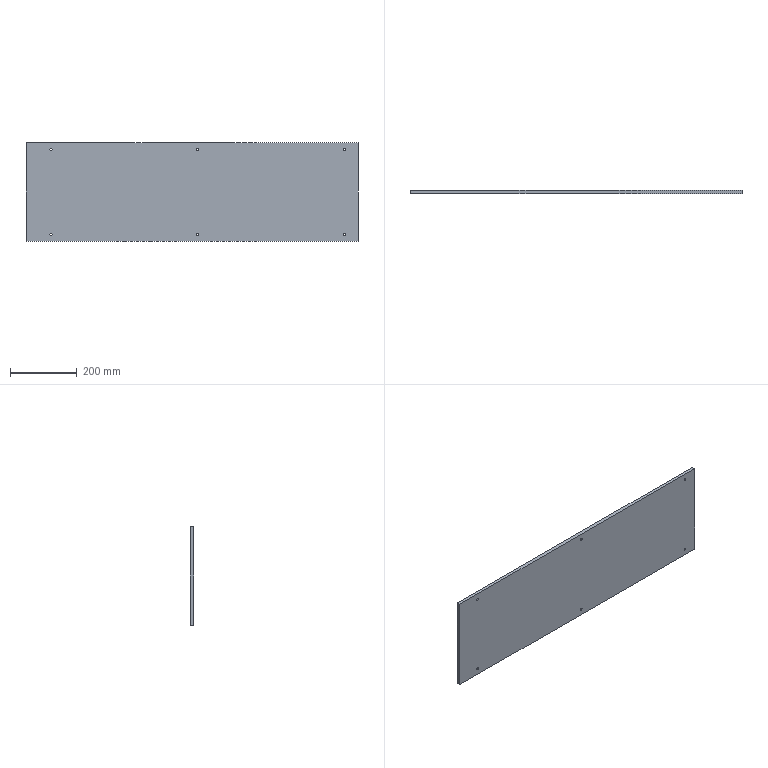Part | SolidWorks | features Extrusion 1, HoleWzd 1 | 1 solid | 30 faces | box 995 x 10 x 295 mm | volume 2932412 mm3 | cone 12 | cylinder 12 | plane 6 | commonest cylinder face diameters 6.6 x12
STEP:
#1=CARTESIAN_POINT('',(75.,6.9,16.7));
#2=VERTEX_POINT('',#1);
#3=CARTESIAN_POINT('',(75.,6.9,23.3));
#4=VERTEX_POINT('',#3);
#5=CARTESIAN_POINT('',(75.,6.9,20.));
#6=DIRECTION('',(0.,1.,0.));
#7=DIRECTION('',(0.,0.,1.));
#8=AXIS2_PLACEMENT_3D('',#5,#6,#7);
#9=CIRCLE('',#8,3.3);
#10=EDGE_CURVE('',#2,#4,#9,.T.);
#11=ORIENTED_EDGE('',*,*,#10,.F.);
#12=CARTESIAN_POINT('',(75.,10.,13.6));
#13=VERTEX_POINT('',#12);
#14=CARTESIAN_POINT('',(75.,10.,13.6));
#15=DIRECTION('',(0.,0.7071,-0.7071));
#16=VECTOR('',#15,1000.);
#17=LINE('',#14,#16);
#18=EDGE_CURVE('',#2,#13,#17,.T.);
#19=ORIENTED_EDGE('',*,*,#18,.T.);
#20=CARTESIAN_POINT('',(75.,10.,26.4));
#21=VERTEX_POINT('',#20);
#22=CARTESIAN_POINT('',(75.,10.,20.));
#23=DIRECTION('',(0.,1.,0.));
#24=DIRECTION('',(0.,0.,1.));
#25=AXIS2_PLACEMENT_3D('',#22,#23,#24);
#26=CIRCLE('',#25,6.4);
#27=EDGE_CURVE('',#13,#21,#26,.T.);
#28=ORIENTED_EDGE('',*,*,#27,.T.);
#29=CARTESIAN_POINT('',(75.,10.,26.4));
#30=DIRECTION('',(0.,0.7071,0.7071));
#31=VECTOR('',#30,1000.);
#32=LINE('',#29,#31);
#33=EDGE_CURVE('',#4,#21,#32,.T.);
#34=ORIENTED_EDGE('',*,*,#33,.F.);
#35=EDGE_LOOP('',(#11,#19,#28,#34));
#36=FACE_OUTER_BOUND('',#35,.T.);
#37=CARTESIAN_POINT('',(75.,10.,20.));
#38=DIRECTION('',(0.,1.,0.));
#39=DIRECTION('',(0.,0.,1.));
#40=AXIS2_PLACEMENT_3D('',#37,#38,#39);
#41=CONICAL_SURFACE('',#40,6.4,0.7854);
#42=ADVANCED_FACE('',(#36),#41,.F.);
#43=CARTESIAN_POINT('',(75.,0.,16.7));
#44=VERTEX_POINT('',#43);
#45=CARTESIAN_POINT('',(75.,0.,23.3));
#46=VERTEX_POINT('',#45);
#47=CARTESIAN_POINT('',(75.,0.,20.));
#48=DIRECTION('',(0.,1.,0.));
#49=DIRECTION('',(0.,0.,1.));
#50=AXIS2_PLACEMENT_3D('',#47,#48,#49);
#51=CIRCLE('',#50,3.3);
#52=EDGE_CURVE('',#44,#46,#51,.T.);
#53=ORIENTED_EDGE('',*,*,#52,.F.);
#54=CARTESIAN_POINT('',(75.,10.,16.7));
#55=DIRECTION('',(0.,1.,0.));
#56=VECTOR('',#55,1000.);
#57=LINE('',#54,#56);
#58=EDGE_CURVE('',#44,#2,#57,.T.);
#59=ORIENTED_EDGE('',*,*,#58,.T.);
#60=ORIENTED_EDGE('',*,*,#10,.T.);
#61=CARTESIAN_POINT('',(75.,10.,23.3));
#62=DIRECTION('',(0.,1.,0.));
#63=VECTOR('',#62,1000.);
#64=LINE('',#61,#63);
#65=EDGE_CURVE('',#46,#4,#64,.T.);
#66=ORIENTED_EDGE('',*,*,#65,.F.);
#67=EDGE_LOOP('',(#53,#59,#60,#66));
#68=FACE_OUTER_BOUND('',#67,.T.);
#69=CARTESIAN_POINT('',(75.,10.,20.));
#70=DIRECTION('',(0.,1.,0.));
#71=DIRECTION('',(0.,0.,1.));
#72=AXIS2_PLACEMENT_3D('',#69,#70,#71);
#73=CYLINDRICAL_SURFACE('',#72,3.3);
#74=ADVANCED_FACE('',(#68),#73,.F.);
#75=CARTESIAN_POINT('',(75.,6.9,271.7));
#76=VERTEX_POINT('',#75);
#77=CARTESIAN_POINT('',(75.,6.9,278.3));
#78=VERTEX_POINT('',#77);
#79=CARTESIAN_POINT('',(75.,6.9,275.));
#80=DIRECTION('',(0.,1.,0.));
#81=DIRECTION('',(0.,0.,1.));
#82=AXIS2_PLACEMENT_3D('',#79,#80,#81);
#83=CIRCLE('',#82,3.3);
#84=EDGE_CURVE('',#76,#78,#83,.T.);
#85=ORIENTED_EDGE('',*,*,#84,.F.);
#86=CARTESIAN_POINT('',(75.,10.,268.6));
#87=VERTEX_POINT('',#86);
#88=CARTESIAN_POINT('',(75.,10.,268.6));
#89=DIRECTION('',(0.,0.7071,-0.7071));
#90=VECTOR('',#89,1000.);
#91=LINE('',#88,#90);
#92=EDGE_CURVE('',#76,#87,#91,.T.);
#93=ORIENTED_EDGE('',*,*,#92,.T.);
#94=CARTESIAN_POINT('',(75.,10.,281.4));
#95=VERTEX_POINT('',#94);
#96=CARTESIAN_POINT('',(75.,10.,275.));
#97=DIRECTION('',(0.,1.,0.));
#98=DIRECTION('',(0.,0.,1.));
#99=AXIS2_PLACEMENT_3D('',#96,#97,#98);
#100=CIRCLE('',#99,6.4);
#101=EDGE_CURVE('',#87,#95,#100,.T.);
#102=ORIENTED_EDGE('',*,*,#101,.T.);
#103=CARTESIAN_POINT('',(75.,10.,281.4));
#104=DIRECTION('',(0.,0.7071,0.7071));
#105=VECTOR('',#104,1000.);
#106=LINE('',#103,#105);
#107=EDGE_CURVE('',#78,#95,#106,.T.);
#108=ORIENTED_EDGE('',*,*,#107,.F.);
#109=EDGE_LOOP('',(#85,#93,#102,#108));
#110=FACE_OUTER_BOUND('',#109,.T.);
#111=CARTESIAN_POINT('',(75.,10.,275.));
#112=DIRECTION('',(0.,1.,0.));
#113=DIRECTION('',(0.,0.,1.));
#114=AXIS2_PLACEMENT_3D('',#111,#112,#113);
#115=CONICAL_SURFACE('',#114,6.4,0.7854);
#116=ADVANCED_FACE('',(#110),#115,.F.);
#117=CARTESIAN_POINT('',(75.,0.,271.7));
#118=VERTEX_POINT('',#117);
#119=CARTESIAN_POINT('',(75.,0.,278.3));
#120=VERTEX_POINT('',#119);
#121=CARTESIAN_POINT('',(75.,0.,275.));
#122=DIRECTION('',(0.,1.,0.));
#123=DIRECTION('',(0.,0.,1.));
#124=AXIS2_PLACEMENT_3D('',#121,#122,#123);
#125=CIRCLE('',#124,3.3);
#126=EDGE_CURVE('',#118,#120,#125,.T.);
#127=ORIENTED_EDGE('',*,*,#126,.F.);
#128=CARTESIAN_POINT('',(75.,10.,271.7));
#129=DIRECTION('',(0.,1.,0.));
#130=VECTOR('',#129,1000.);
#131=LINE('',#128,#130);
#132=EDGE_CURVE('',#118,#76,#131,.T.);
#133=ORIENTED_EDGE('',*,*,#132,.T.);
#134=ORIENTED_EDGE('',*,*,#84,.T.);
#135=CARTESIAN_POINT('',(75.,10.,278.3));
#136=DIRECTION('',(0.,1.,0.));
#137=VECTOR('',#136,1000.);
#138=LINE('',#135,#137);
#139=EDGE_CURVE('',#120,#78,#138,.T.);
#140=ORIENTED_EDGE('',*,*,#139,.F.);
#141=EDGE_LOOP('',(#127,#133,#134,#140));
#142=FACE_OUTER_BOUND('',#141,.T.);
#143=CARTESIAN_POINT('',(75.,10.,275.));
#144=DIRECTION('',(0.,1.,0.));
#145=DIRECTION('',(0.,0.,1.));
#146=AXIS2_PLACEMENT_3D('',#143,#144,#145);
#147=CYLINDRICAL_SURFACE('',#146,3.3);
#148=ADVANCED_FACE('',(#142),#147,.F.);
#149=CARTESIAN_POINT('',(515.,6.9,16.7));
#150=VERTEX_POINT('',#149);
#151=CARTESIAN_POINT('',(515.,6.9,23.3));
#152=VERTEX_POINT('',#151);
#153=CARTESIAN_POINT('',(515.,6.9,20.));
#154=DIRECTION('',(0.,1.,0.));
#155=DIRECTION('',(0.,0.,1.));
#156=AXIS2_PLACEMENT_3D('',#153,#154,#155);
#157=CIRCLE('',#156,3.3);
#158=EDGE_CURVE('',#150,#152,#157,.T.);
#159=ORIENTED_EDGE('',*,*,#158,.F.);
#160=CARTESIAN_POINT('',(515.,10.,13.6));
#161=VERTEX_POINT('',#160);
#162=CARTESIAN_POINT('',(515.,10.,13.6));
#163=DIRECTION('',(0.,0.7071,-0.7071));
#164=VECTOR('',#163,1000.);
#165=LINE('',#162,#164);
#166=EDGE_CURVE('',#150,#161,#165,.T.);
#167=ORIENTED_EDGE('',*,*,#166,.T.);
#168=CARTESIAN_POINT('',(515.,10.,26.4));
#169=VERTEX_POINT('',#168);
#170=CARTESIAN_POINT('',(515.,10.,20.));
#171=DIRECTION('',(0.,1.,0.));
#172=DIRECTION('',(0.,0.,1.));
#173=AXIS2_PLACEMENT_3D('',#170,#171,#172);
#174=CIRCLE('',#173,6.4);
#175=EDGE_CURVE('',#161,#169,#174,.T.);
#176=ORIENTED_EDGE('',*,*,#175,.T.);
#177=CARTESIAN_POINT('',(515.,10.,26.4));
#178=DIRECTION('',(0.,0.7071,0.7071));
#179=VECTOR('',#178,1000.);
#180=LINE('',#177,#179);
#181=EDGE_CURVE('',#152,#169,#180,.T.);
#182=ORIENTED_EDGE('',*,*,#181,.F.);
#183=EDGE_LOOP('',(#159,#167,#176,#182));
#184=FACE_OUTER_BOUND('',#183,.T.);
#185=CARTESIAN_POINT('',(515.,10.,20.));
#186=DIRECTION('',(0.,1.,0.));
#187=DIRECTION('',(0.,0.,1.));
#188=AXIS2_PLACEMENT_3D('',#185,#186,#187);
#189=CONICAL_SURFACE('',#188,6.4,0.7854);
#190=ADVANCED_FACE('',(#184),#189,.F.);
#191=CARTESIAN_POINT('',(515.,0.,16.7));
#192=VERTEX_POINT('',#191);
#193=CARTESIAN_POINT('',(515.,0.,23.3));
#194=VERTEX_POINT('',#193);
#195=CARTESIAN_POINT('',(515.,0.,20.));
#196=DIRECTION('',(0.,1.,0.));
#197=DIRECTION('',(0.,0.,1.));
#198=AXIS2_PLACEMENT_3D('',#195,#196,#197);
#199=CIRCLE('',#198,3.3);
#200=EDGE_CURVE('',#192,#194,#199,.T.);
#201=ORIENTED_EDGE('',*,*,#200,.F.);
#202=CARTESIAN_POINT('',(515.,10.,16.7));
#203=DIRECTION('',(0.,1.,0.));
#204=VECTOR('',#203,1000.);
#205=LINE('',#202,#204);
#206=EDGE_CURVE('',#192,#150,#205,.T.);
#207=ORIENTED_EDGE('',*,*,#206,.T.);
#208=ORIENTED_EDGE('',*,*,#158,.T.);
#209=CARTESIAN_POINT('',(515.,10.,23.3));
#210=DIRECTION('',(0.,1.,0.));
#211=VECTOR('',#210,1000.);
#212=LINE('',#209,#211);
#213=EDGE_CURVE('',#194,#152,#212,.T.);
#214=ORIENTED_EDGE('',*,*,#213,.F.);
#215=EDGE_LOOP('',(#201,#207,#208,#214));
#216=FACE_OUTER_BOUND('',#215,.T.);
#217=CARTESIAN_POINT('',(515.,10.,20.));
#218=DIRECTION('',(0.,1.,0.));
#219=DIRECTION('',(0.,0.,1.));
#220=AXIS2_PLACEMENT_3D('',#217,#218,#219);
#221=CYLINDRICAL_SURFACE('',#220,3.3);
#222=ADVANCED_FACE('',(#216),#221,.F.);
#223=CARTESIAN_POINT('',(515.,6.9,271.7));
#224=VERTEX_POINT('',#223);
#225=CARTESIAN_POINT('',(515.,6.9,278.3));
#226=VERTEX_POINT('',#225);
#227=CARTESIAN_POINT('',(515.,6.9,275.));
#228=DIRECTION('',(0.,1.,0.));
#229=DIRECTION('',(0.,0.,1.));
#230=AXIS2_PLACEMENT_3D('',#227,#228,#229);
#231=CIRCLE('',#230,3.3);
#232=EDGE_CURVE('',#224,#226,#231,.T.);
#233=ORIENTED_EDGE('',*,*,#232,.F.);
#234=CARTESIAN_POINT('',(515.,10.,268.6));
#235=VERTEX_POINT('',#234);
#236=CARTESIAN_POINT('',(515.,10.,268.6));
#237=DIRECTION('',(0.,0.7071,-0.7071));
#238=VECTOR('',#237,1000.);
#239=LINE('',#236,#238);
#240=EDGE_CURVE('',#224,#235,#239,.T.);
#241=ORIENTED_EDGE('',*,*,#240,.T.);
#242=CARTESIAN_POINT('',(515.,10.,281.4));
#243=VERTEX_POINT('',#242);
#244=CARTESIAN_POINT('',(515.,10.,275.));
#245=DIRECTION('',(0.,1.,0.));
#246=DIRECTION('',(0.,0.,1.));
#247=AXIS2_PLACEMENT_3D('',#244,#245,#246);
#248=CIRCLE('',#247,6.4);
#249=EDGE_CURVE('',#235,#243,#248,.T.);
#250=ORIENTED_EDGE('',*,*,#249,.T.);
#251=CARTESIAN_POINT('',(515.,10.,281.4));
#252=DIRECTION('',(0.,0.7071,0.7071));
#253=VECTOR('',#252,1000.);
#254=LINE('',#251,#253);
#255=EDGE_CURVE('',#226,#243,#254,.T.);
#256=ORIENTED_EDGE('',*,*,#255,.F.);
#257=EDGE_LOOP('',(#233,#241,#250,#256));
#258=FACE_OUTER_BOUND('',#257,.T.);
#259=CARTESIAN_POINT('',(515.,10.,275.));
#260=DIRECTION('',(0.,1.,0.));
#261=DIRECTION('',(0.,0.,1.));
#262=AXIS2_PLACEMENT_3D('',#259,#260,#261);
#263=CONICAL_SURFACE('',#262,6.4,0.7854);
#264=ADVANCED_FACE('',(#258),#263,.F.);
#265=CARTESIAN_POINT('',(515.,0.,271.7));
#266=VERTEX_POINT('',#265);
#267=CARTESIAN_POINT('',(515.,0.,278.3));
#268=VERTEX_POINT('',#267);
#269=CARTESIAN_POINT('',(515.,0.,275.));
#270=DIRECTION('',(0.,1.,0.));
#271=DIRECTION('',(0.,0.,1.));
#272=AXIS2_PLACEMENT_3D('',#269,#270,#271);
#273=CIRCLE('',#272,3.3);
#274=EDGE_CURVE('',#266,#268,#273,.T.);
#275=ORIENTED_EDGE('',*,*,#274,.F.);
#276=CARTESIAN_POINT('',(515.,10.,271.7));
#277=DIRECTION('',(0.,1.,0.));
#278=VECTOR('',#277,1000.);
#279=LINE('',#276,#278);
#280=EDGE_CURVE('',#266,#224,#279,.T.);
#281=ORIENTED_EDGE('',*,*,#280,.T.);
#282=ORIENTED_EDGE('',*,*,#232,.T.);
#283=CARTESIAN_POINT('',(515.,10.,278.3));
#284=DIRECTION('',(0.,1.,0.));
#285=VECTOR('',#284,1000.);
#286=LINE('',#283,#285);
#287=EDGE_CURVE('',#268,#226,#286,.T.);
#288=ORIENTED_EDGE('',*,*,#287,.F.);
#289=EDGE_LOOP('',(#275,#281,#282,#288));
#290=FACE_OUTER_BOUND('',#289,.T.);
#291=CARTESIAN_POINT('',(515.,10.,275.));
#292=DIRECTION('',(0.,1.,0.));
#293=DIRECTION('',(0.,0.,1.));
#294=AXIS2_PLACEMENT_3D('',#291,#292,#293);
#295=CYLINDRICAL_SURFACE('',#294,3.3);
#296=ADVANCED_FACE('',(#290),#295,.F.);
#297=CARTESIAN_POINT('',(955.,6.9,271.7));
#298=VERTEX_POINT('',#297);
#299=CARTESIAN_POINT('',(955.,6.9,278.3));
#300=VERTEX_POINT('',#299);
#301=CARTESIAN_POINT('',(955.,6.9,275.));
#302=DIRECTION('',(0.,1.,0.));
#303=DIRECTION('',(0.,0.,1.));
#304=AXIS2_PLACEMENT_3D('',#301,#302,#303);
#305=CIRCLE('',#304,3.3);
#306=EDGE_CURVE('',#298,#300,#305,.T.);
#307=ORIENTED_EDGE('',*,*,#306,.F.);
#308=CARTESIAN_POINT('',(955.,10.,268.6));
#309=VERTEX_POINT('',#308);
#310=CARTESIAN_POINT('',(955.,10.,268.6));
#311=DIRECTION('',(0.,0.7071,-0.7071));
#312=VECTOR('',#311,1000.);
#313=LINE('',#310,#312);
#314=EDGE_CURVE('',#298,#309,#313,.T.);
#315=ORIENTED_EDGE('',*,*,#314,.T.);
#316=CARTESIAN_POINT('',(955.,10.,281.4));
#317=VERTEX_POINT('',#316);
#318=CARTESIAN_POINT('',(955.,10.,275.));
#319=DIRECTION('',(0.,1.,0.));
#320=DIRECTION('',(0.,0.,1.));
#321=AXIS2_PLACEMENT_3D('',#318,#319,#320);
#322=CIRCLE('',#321,6.4);
#323=EDGE_CURVE('',#309,#317,#322,.T.);
#324=ORIENTED_EDGE('',*,*,#323,.T.);
#325=CARTESIAN_POINT('',(955.,10.,281.4));
#326=DIRECTION('',(0.,0.7071,0.7071));
#327=VECTOR('',#326,1000.);
#328=LINE('',#325,#327);
#329=EDGE_CURVE('',#300,#317,#328,.T.);
#330=ORIENTED_EDGE('',*,*,#329,.F.);
#331=EDGE_LOOP('',(#307,#315,#324,#330));
#332=FACE_OUTER_BOUND('',#331,.T.);
#333=CARTESIAN_POINT('',(955.,10.,275.));
#334=DIRECTION('',(0.,1.,0.));
#335=DIRECTION('',(0.,0.,1.));
#336=AXIS2_PLACEMENT_3D('',#333,#334,#335);
#337=CONICAL_SURFACE('',#336,6.4,0.7854);
#338=ADVANCED_FACE('',(#332),#337,.F.);
#339=CARTESIAN_POINT('',(955.,0.,271.7));
#340=VERTEX_POINT('',#339);
#341=CARTESIAN_POINT('',(955.,0.,278.3));
#342=VERTEX_POINT('',#341);
#343=CARTESIAN_POINT('',(955.,0.,275.));
#344=DIRECTION('',(0.,1.,0.));
#345=DIRECTION('',(0.,0.,1.));
#346=AXIS2_PLACEMENT_3D('',#343,#344,#345);
#347=CIRCLE('',#346,3.3);
#348=EDGE_CURVE('',#340,#342,#347,.T.);
#349=ORIENTED_EDGE('',*,*,#348,.F.);
#350=CARTESIAN_POINT('',(955.,10.,271.7));
#351=DIRECTION('',(0.,1.,0.));
#352=VECTOR('',#351,1000.);
#353=LINE('',#350,#352);
#354=EDGE_CURVE('',#340,#298,#353,.T.);
#355=ORIENTED_EDGE('',*,*,#354,.T.);
#356=ORIENTED_EDGE('',*,*,#306,.T.);
#357=CARTESIAN_POINT('',(955.,10.,278.3));
#358=DIRECTION('',(0.,1.,0.));
#359=VECTOR('',#358,1000.);
#360=LINE('',#357,#359);
#361=EDGE_CURVE('',#342,#300,#360,.T.);
#362=ORIENTED_EDGE('',*,*,#361,.F.);
#363=EDGE_LOOP('',(#349,#355,#356,#362));
#364=FACE_OUTER_BOUND('',#363,.T.);
#365=CARTESIAN_POINT('',(955.,10.,275.));
#366=DIRECTION('',(0.,1.,0.));
#367=DIRECTION('',(0.,0.,1.));
#368=AXIS2_PLACEMENT_3D('',#365,#366,#367);
#369=CYLINDRICAL_SURFACE('',#368,3.3);
#370=ADVANCED_FACE('',(#364),#369,.F.);
#371=CARTESIAN_POINT('',(955.,6.9,16.7));
#372=VERTEX_POINT('',#371);
#373=CARTESIAN_POINT('',(955.,6.9,23.3));
#374=VERTEX_POINT('',#373);
#375=CARTESIAN_POINT('',(955.,6.9,20.));
#376=DIRECTION('',(0.,1.,0.));
#377=DIRECTION('',(0.,0.,1.));
#378=AXIS2_PLACEMENT_3D('',#375,#376,#377);
#379=CIRCLE('',#378,3.3);
#380=EDGE_CURVE('',#372,#374,#379,.T.);
#381=ORIENTED_EDGE('',*,*,#380,.F.);
#382=CARTESIAN_POINT('',(955.,10.,13.6));
#383=VERTEX_POINT('',#382);
#384=CARTESIAN_POINT('',(955.,10.,13.6));
#385=DIRECTION('',(0.,0.7071,-0.7071));
#386=VECTOR('',#385,1000.);
#387=LINE('',#384,#386);
#388=EDGE_CURVE('',#372,#383,#387,.T.);
#389=ORIENTED_EDGE('',*,*,#388,.T.);
#390=CARTESIAN_POINT('',(955.,10.,26.4));
#391=VERTEX_POINT('',#390);
#392=CARTESIAN_POINT('',(955.,10.,20.));
#393=DIRECTION('',(0.,1.,0.));
#394=DIRECTION('',(0.,0.,1.));
#395=AXIS2_PLACEMENT_3D('',#392,#393,#394);
#396=CIRCLE('',#395,6.4);
#397=EDGE_CURVE('',#383,#391,#396,.T.);
#398=ORIENTED_EDGE('',*,*,#397,.T.);
#399=CARTESIAN_POINT('',(955.,10.,26.4));
#400=DIRECTION('',(0.,0.7071,0.7071));
#401=VECTOR('',#400,1000.);
#402=LINE('',#399,#401);
#403=EDGE_CURVE('',#374,#391,#402,.T.);
#404=ORIENTED_EDGE('',*,*,#403,.F.);
#405=EDGE_LOOP('',(#381,#389,#398,#404));
#406=FACE_OUTER_BOUND('',#405,.T.);
#407=CARTESIAN_POINT('',(955.,10.,20.));
#408=DIRECTION('',(0.,1.,0.));
#409=DIRECTION('',(0.,0.,1.));
#410=AXIS2_PLACEMENT_3D('',#407,#408,#409);
#411=CONICAL_SURFACE('',#410,6.4,0.7854);
#412=ADVANCED_FACE('',(#406),#411,.F.);
#413=CARTESIAN_POINT('',(955.,0.,16.7));
#414=VERTEX_POINT('',#413);
#415=CARTESIAN_POINT('',(955.,0.,23.3));
#416=VERTEX_POINT('',#415);
#417=CARTESIAN_POINT('',(955.,0.,20.));
#418=DIRECTION('',(0.,1.,0.));
#419=DIRECTION('',(0.,0.,1.));
#420=AXIS2_PLACEMENT_3D('',#417,#418,#419);
#421=CIRCLE('',#420,3.3);
#422=EDGE_CURVE('',#414,#416,#421,.T.);
#423=ORIENTED_EDGE('',*,*,#422,.F.);
#424=CARTESIAN_POINT('',(955.,10.,16.7));
#425=DIRECTION('',(0.,1.,0.));
#426=VECTOR('',#425,1000.);
#427=LINE('',#424,#426);
#428=EDGE_CURVE('',#414,#372,#427,.T.);
#429=ORIENTED_EDGE('',*,*,#428,.T.);
#430=ORIENTED_EDGE('',*,*,#380,.T.);
#431=CARTESIAN_POINT('',(955.,10.,23.3));
#432=DIRECTION('',(0.,1.,0.));
#433=VECTOR('',#432,1000.);
#434=LINE('',#431,#433);
#435=EDGE_CURVE('',#416,#374,#434,.T.);
#436=ORIENTED_EDGE('',*,*,#435,.F.);
#437=EDGE_LOOP('',(#423,#429,#430,#436));
#438=FACE_OUTER_BOUND('',#437,.T.);
#439=CARTESIAN_POINT('',(955.,10.,20.));
#440=DIRECTION('',(0.,1.,0.));
#441=DIRECTION('',(0.,0.,1.));
#442=AXIS2_PLACEMENT_3D('',#439,#440,#441);
#443=CYLINDRICAL_SURFACE('',#442,3.3);
#444=ADVANCED_FACE('',(#438),#443,.F.);
#445=CARTESIAN_POINT('',(0.,0.,0.));
#446=VERTEX_POINT('',#445);
#447=CARTESIAN_POINT('',(0.,0.,295.));
#448=VERTEX_POINT('',#447);
#449=CARTESIAN_POINT('',(0.,0.,0.));
#450=DIRECTION('',(0.,0.,1.));
#451=VECTOR('',#450,1000.);
#452=LINE('',#449,#451);
#453=EDGE_CURVE('',#446,#448,#452,.T.);
#454=ORIENTED_EDGE('',*,*,#453,.T.);
#455=CARTESIAN_POINT('',(0.,10.,295.));
#456=VERTEX_POINT('',#455);
#457=CARTESIAN_POINT('',(0.,10.,295.));
#458=DIRECTION('',(0.,-1.,0.));
#459=VECTOR('',#458,1000.);
#460=LINE('',#457,#459);
#461=EDGE_CURVE('',#456,#448,#460,.T.);
#462=ORIENTED_EDGE('',*,*,#461,.F.);
#463=CARTESIAN_POINT('',(0.,10.,0.));
#464=VERTEX_POINT('',#463);
#465=CARTESIAN_POINT('',(0.,10.,0.));
#466=DIRECTION('',(0.,0.,1.));
#467=VECTOR('',#466,1000.);
#468=LINE('',#465,#467);
#469=EDGE_CURVE('',#464,#456,#468,.T.);
#470=ORIENTED_EDGE('',*,*,#469,.F.);
#471=CARTESIAN_POINT('',(0.,10.,0.));
#472=DIRECTION('',(0.,-1.,0.));
#473=VECTOR('',#472,1000.);
#474=LINE('',#471,#473);
#475=EDGE_CURVE('',#464,#446,#474,.T.);
#476=ORIENTED_EDGE('',*,*,#475,.T.);
#477=EDGE_LOOP('',(#454,#462,#470,#476));
#478=FACE_OUTER_BOUND('',#477,.T.);
#479=CARTESIAN_POINT('',(0.,10.,0.));
#480=DIRECTION('',(1.,0.,0.));
#481=DIRECTION('',(0.,0.,-1.));
#482=AXIS2_PLACEMENT_3D('',#479,#480,#481);
#483=PLANE('',#482);
#484=ADVANCED_FACE('',(#478),#483,.F.);
#485=CARTESIAN_POINT('',(995.,0.,295.));
#486=VERTEX_POINT('',#485);
#487=CARTESIAN_POINT('',(0.,0.,295.));
#488=DIRECTION('',(1.,0.,0.));
#489=VECTOR('',#488,1000.);
#490=LINE('',#487,#489);
#491=EDGE_CURVE('',#448,#486,#490,.T.);
#492=ORIENTED_EDGE('',*,*,#491,.T.);
#493=CARTESIAN_POINT('',(995.,10.,295.));
#494=VERTEX_POINT('',#493);
#495=CARTESIAN_POINT('',(995.,10.,295.));
#496=DIRECTION('',(0.,-1.,0.));
#497=VECTOR('',#496,1000.);
#498=LINE('',#495,#497);
#499=EDGE_CURVE('',#494,#486,#498,.T.);
#500=ORIENTED_EDGE('',*,*,#499,.F.);
#501=CARTESIAN_POINT('',(0.,10.,295.));
#502=DIRECTION('',(1.,0.,0.));
#503=VECTOR('',#502,1000.);
#504=LINE('',#501,#503);
#505=EDGE_CURVE('',#456,#494,#504,.T.);
#506=ORIENTED_EDGE('',*,*,#505,.F.);
#507=ORIENTED_EDGE('',*,*,#461,.T.);
#508=EDGE_LOOP('',(#492,#500,#506,#507));
#509=FACE_OUTER_BOUND('',#508,.T.);
#510=CARTESIAN_POINT('',(0.,10.,295.));
#511=DIRECTION('',(0.,0.,-1.));
#512=DIRECTION('',(-1.,0.,0.));
#513=AXIS2_PLACEMENT_3D('',#510,#511,#512);
#514=PLANE('',#513);
#515=ADVANCED_FACE('',(#509),#514,.F.);
#516=CARTESIAN_POINT('',(995.,0.,0.));
#517=VERTEX_POINT('',#516);
#518=CARTESIAN_POINT('',(995.,0.,0.));
#519=DIRECTION('',(0.,0.,-1.));
#520=VECTOR('',#519,1000.);
#521=LINE('',#518,#520);
#522=EDGE_CURVE('',#486,#517,#521,.T.);
#523=ORIENTED_EDGE('',*,*,#522,.T.);
#524=CARTESIAN_POINT('',(995.,10.,0.));
#525=VERTEX_POINT('',#524);
#526=CARTESIAN_POINT('',(995.,10.,0.));
#527=DIRECTION('',(0.,-1.,0.));
#528=VECTOR('',#527,1000.);
#529=LINE('',#526,#528);
#530=EDGE_CURVE('',#525,#517,#529,.T.);
#531=ORIENTED_EDGE('',*,*,#530,.F.);
#532=CARTESIAN_POINT('',(995.,10.,0.));
#533=DIRECTION('',(0.,0.,-1.));
#534=VECTOR('',#533,1000.);
#535=LINE('',#532,#534);
#536=EDGE_CURVE('',#494,#525,#535,.T.);
#537=ORIENTED_EDGE('',*,*,#536,.F.);
#538=ORIENTED_EDGE('',*,*,#499,.T.);
#539=EDGE_LOOP('',(#523,#531,#537,#538));
#540=FACE_OUTER_BOUND('',#539,.T.);
#541=CARTESIAN_POINT('',(995.,10.,0.));
#542=DIRECTION('',(-1.,0.,0.));
#543=DIRECTION('',(0.,0.,1.));
#544=AXIS2_PLACEMENT_3D('',#541,#542,#543);
#545=PLANE('',#544);
#546=ADVANCED_FACE('',(#540),#545,.F.);
#547=CARTESIAN_POINT('',(0.,0.,0.));
#548=DIRECTION('',(-1.,0.,0.));
#549=VECTOR('',#548,1000.);
#550=LINE('',#547,#549);
#551=EDGE_CURVE('',#517,#446,#550,.T.);
#552=ORIENTED_EDGE('',*,*,#551,.T.);
#553=ORIENTED_EDGE('',*,*,#475,.F.);
#554=CARTESIAN_POINT('',(0.,10.,0.));
#555=DIRECTION('',(-1.,0.,0.));
#556=VECTOR('',#555,1000.);
#557=LINE('',#554,#556);
#558=EDGE_CURVE('',#525,#464,#557,.T.);
#559=ORIENTED_EDGE('',*,*,#558,.F.);
#560=ORIENTED_EDGE('',*,*,#530,.T.);
#561=EDGE_LOOP('',(#552,#553,#559,#560));
#562=FACE_OUTER_BOUND('',#561,.T.);
#563=CARTESIAN_POINT('',(0.,10.,0.));
#564=DIRECTION('',(0.,0.,1.));
#565=DIRECTION('',(1.,0.,0.));
#566=AXIS2_PLACEMENT_3D('',#563,#564,#565);
#567=PLANE('',#566);
#568=ADVANCED_FACE('',(#562),#567,.F.);
#569=CARTESIAN_POINT('',(75.,10.,20.));
#570=DIRECTION('',(0.,1.,0.));
#571=DIRECTION('',(0.,0.,1.));
#572=AXIS2_PLACEMENT_3D('',#569,#570,#571);
#573=CIRCLE('',#572,6.4);
#574=EDGE_CURVE('',#21,#13,#573,.T.);
#575=ORIENTED_EDGE('',*,*,#574,.F.);
#576=ORIENTED_EDGE('',*,*,#27,.F.);
#577=EDGE_LOOP('',(#575,#576));
#578=FACE_BOUND('',#577,.T.);
#579=CARTESIAN_POINT('',(75.,10.,275.));
#580=DIRECTION('',(0.,1.,0.));
#581=DIRECTION('',(0.,0.,1.));
#582=AXIS2_PLACEMENT_3D('',#579,#580,#581);
#583=CIRCLE('',#582,6.4);
#584=EDGE_CURVE('',#95,#87,#583,.T.);
#585=ORIENTED_EDGE('',*,*,#584,.F.);
#586=ORIENTED_EDGE('',*,*,#101,.F.);
#587=EDGE_LOOP('',(#585,#586));
#588=FACE_BOUND('',#587,.T.);
#589=CARTESIAN_POINT('',(515.,10.,20.));
#590=DIRECTION('',(0.,1.,0.));
#591=DIRECTION('',(0.,0.,1.));
#592=AXIS2_PLACEMENT_3D('',#589,#590,#591);
#593=CIRCLE('',#592,6.4);
#594=EDGE_CURVE('',#169,#161,#593,.T.);
#595=ORIENTED_EDGE('',*,*,#594,.F.);
#596=ORIENTED_EDGE('',*,*,#175,.F.);
#597=EDGE_LOOP('',(#595,#596));
#598=FACE_BOUND('',#597,.T.);
#599=CARTESIAN_POINT('',(515.,10.,275.));
#600=DIRECTION('',(0.,1.,0.));
#601=DIRECTION('',(0.,0.,1.));
#602=AXIS2_PLACEMENT_3D('',#599,#600,#601);
#603=CIRCLE('',#602,6.4);
#604=EDGE_CURVE('',#243,#235,#603,.T.);
#605=ORIENTED_EDGE('',*,*,#604,.F.);
#606=ORIENTED_EDGE('',*,*,#249,.F.);
#607=EDGE_LOOP('',(#605,#606));
#608=FACE_BOUND('',#607,.T.);
#609=CARTESIAN_POINT('',(955.,10.,275.));
#610=DIRECTION('',(0.,1.,0.));
#611=DIRECTION('',(0.,0.,1.));
#612=AXIS2_PLACEMENT_3D('',#609,#610,#611);
#613=CIRCLE('',#612,6.4);
#614=EDGE_CURVE('',#317,#309,#613,.T.);
#615=ORIENTED_EDGE('',*,*,#614,.F.);
#616=ORIENTED_EDGE('',*,*,#323,.F.);
#617=EDGE_LOOP('',(#615,#616));
#618=FACE_BOUND('',#617,.T.);
#619=CARTESIAN_POINT('',(955.,10.,20.));
#620=DIRECTION('',(0.,1.,0.));
#621=DIRECTION('',(0.,0.,1.));
#622=AXIS2_PLACEMENT_3D('',#619,#620,#621);
#623=CIRCLE('',#622,6.4);
#624=EDGE_CURVE('',#391,#383,#623,.T.);
#625=ORIENTED_EDGE('',*,*,#624,.F.);
#626=ORIENTED_EDGE('',*,*,#397,.F.);
#627=EDGE_LOOP('',(#625,#626));
#628=FACE_BOUND('',#627,.T.);
#629=ORIENTED_EDGE('',*,*,#469,.T.);
#630=ORIENTED_EDGE('',*,*,#505,.T.);
#631=ORIENTED_EDGE('',*,*,#536,.T.);
#632=ORIENTED_EDGE('',*,*,#558,.T.);
#633=EDGE_LOOP('',(#629,#630,#631,#632));
#634=FACE_OUTER_BOUND('',#633,.T.);
#635=CARTESIAN_POINT('',(0.,10.,0.));
#636=DIRECTION('',(0.,1.,0.));
#637=DIRECTION('',(0.,0.,1.));
#638=AXIS2_PLACEMENT_3D('',#635,#636,#637);
#639=PLANE('',#638);
#640=ADVANCED_FACE('',(#578,#588,#598,#608,#618,#628,#634),#639,.T.);
#641=CARTESIAN_POINT('',(75.,0.,20.));
#642=DIRECTION('',(0.,1.,0.));
#643=DIRECTION('',(0.,0.,1.));
#644=AXIS2_PLACEMENT_3D('',#641,#642,#643);
#645=CIRCLE('',#644,3.3);
#646=EDGE_CURVE('',#46,#44,#645,.T.);
#647=ORIENTED_EDGE('',*,*,#646,.T.);
#648=ORIENTED_EDGE('',*,*,#52,.T.);
#649=EDGE_LOOP('',(#647,#648));
#650=FACE_BOUND('',#649,.T.);
#651=CARTESIAN_POINT('',(75.,0.,275.));
#652=DIRECTION('',(0.,1.,0.));
#653=DIRECTION('',(0.,0.,1.));
#654=AXIS2_PLACEMENT_3D('',#651,#652,#653);
#655=CIRCLE('',#654,3.3);
#656=EDGE_CURVE('',#120,#118,#655,.T.);
#657=ORIENTED_EDGE('',*,*,#656,.T.);
#658=ORIENTED_EDGE('',*,*,#126,.T.);
#659=EDGE_LOOP('',(#657,#658));
#660=FACE_BOUND('',#659,.T.);
#661=CARTESIAN_POINT('',(515.,0.,20.));
#662=DIRECTION('',(0.,1.,0.));
#663=DIRECTION('',(0.,0.,1.));
#664=AXIS2_PLACEMENT_3D('',#661,#662,#663);
#665=CIRCLE('',#664,3.3);
#666=EDGE_CURVE('',#194,#192,#665,.T.);
#667=ORIENTED_EDGE('',*,*,#666,.T.);
#668=ORIENTED_EDGE('',*,*,#200,.T.);
#669=EDGE_LOOP('',(#667,#668));
#670=FACE_BOUND('',#669,.T.);
#671=CARTESIAN_POINT('',(515.,0.,275.));
#672=DIRECTION('',(0.,1.,0.));
#673=DIRECTION('',(0.,0.,1.));
#674=AXIS2_PLACEMENT_3D('',#671,#672,#673);
#675=CIRCLE('',#674,3.3);
#676=EDGE_CURVE('',#268,#266,#675,.T.);
#677=ORIENTED_EDGE('',*,*,#676,.T.);
#678=ORIENTED_EDGE('',*,*,#274,.T.);
#679=EDGE_LOOP('',(#677,#678));
#680=FACE_BOUND('',#679,.T.);
#681=CARTESIAN_POINT('',(955.,0.,275.));
#682=DIRECTION('',(0.,1.,0.));
#683=DIRECTION('',(0.,0.,1.));
#684=AXIS2_PLACEMENT_3D('',#681,#682,#683);
#685=CIRCLE('',#684,3.3);
#686=EDGE_CURVE('',#342,#340,#685,.T.);
#687=ORIENTED_EDGE('',*,*,#686,.T.);
#688=ORIENTED_EDGE('',*,*,#348,.T.);
#689=EDGE_LOOP('',(#687,#688));
#690=FACE_BOUND('',#689,.T.);
#691=CARTESIAN_POINT('',(955.,0.,20.));
#692=DIRECTION('',(0.,1.,0.));
#693=DIRECTION('',(0.,0.,1.));
#694=AXIS2_PLACEMENT_3D('',#691,#692,#693);
#695=CIRCLE('',#694,3.3);
#696=EDGE_CURVE('',#416,#414,#695,.T.);
#697=ORIENTED_EDGE('',*,*,#696,.T.);
#698=ORIENTED_EDGE('',*,*,#422,.T.);
#699=EDGE_LOOP('',(#697,#698));
#700=FACE_BOUND('',#699,.T.);
#701=ORIENTED_EDGE('',*,*,#453,.F.);
#702=ORIENTED_EDGE('',*,*,#551,.F.);
#703=ORIENTED_EDGE('',*,*,#522,.F.);
#704=ORIENTED_EDGE('',*,*,#491,.F.);
#705=EDGE_LOOP('',(#701,#702,#703,#704));
#706=FACE_OUTER_BOUND('',#705,.T.);
#707=CARTESIAN_POINT('',(0.,0.,0.));
#708=DIRECTION('',(0.,1.,0.));
#709=DIRECTION('',(0.,0.,1.));
#710=AXIS2_PLACEMENT_3D('',#707,#708,#709);
#711=PLANE('',#710);
#712=ADVANCED_FACE('',(#650,#660,#670,#680,#690,#700,#706),#711,.F.);
#713=ORIENTED_EDGE('',*,*,#428,.F.);
#714=ORIENTED_EDGE('',*,*,#696,.F.);
#715=ORIENTED_EDGE('',*,*,#435,.T.);
#716=CARTESIAN_POINT('',(955.,6.9,20.));
#717=DIRECTION('',(0.,1.,0.));
#718=DIRECTION('',(0.,0.,1.));
#719=AXIS2_PLACEMENT_3D('',#716,#717,#718);
#720=CIRCLE('',#719,3.3);
#721=EDGE_CURVE('',#374,#372,#720,.T.);
#722=ORIENTED_EDGE('',*,*,#721,.T.);
#723=EDGE_LOOP('',(#713,#714,#715,#722));
#724=FACE_OUTER_BOUND('',#723,.T.);
#725=CARTESIAN_POINT('',(955.,10.,20.));
#726=DIRECTION('',(0.,1.,0.));
#727=DIRECTION('',(0.,0.,1.));
#728=AXIS2_PLACEMENT_3D('',#725,#726,#727);
#729=CYLINDRICAL_SURFACE('',#728,3.3);
#730=ADVANCED_FACE('',(#724),#729,.F.);
#731=ORIENTED_EDGE('',*,*,#388,.F.);
#732=ORIENTED_EDGE('',*,*,#721,.F.);
#733=ORIENTED_EDGE('',*,*,#403,.T.);
#734=ORIENTED_EDGE('',*,*,#624,.T.);
#735=EDGE_LOOP('',(#731,#732,#733,#734));
#736=FACE_OUTER_BOUND('',#735,.T.);
#737=CARTESIAN_POINT('',(955.,10.,20.));
#738=DIRECTION('',(0.,1.,0.));
#739=DIRECTION('',(0.,0.,1.));
#740=AXIS2_PLACEMENT_3D('',#737,#738,#739);
#741=CONICAL_SURFACE('',#740,6.4,0.7854);
#742=ADVANCED_FACE('',(#736),#741,.F.);
#743=ORIENTED_EDGE('',*,*,#354,.F.);
#744=ORIENTED_EDGE('',*,*,#686,.F.);
#745=ORIENTED_EDGE('',*,*,#361,.T.);
#746=CARTESIAN_POINT('',(955.,6.9,275.));
#747=DIRECTION('',(0.,1.,0.));
#748=DIRECTION('',(0.,0.,1.));
#749=AXIS2_PLACEMENT_3D('',#746,#747,#748);
#750=CIRCLE('',#749,3.3);
#751=EDGE_CURVE('',#300,#298,#750,.T.);
#752=ORIENTED_EDGE('',*,*,#751,.T.);
#753=EDGE_LOOP('',(#743,#744,#745,#752));
#754=FACE_OUTER_BOUND('',#753,.T.);
#755=CARTESIAN_POINT('',(955.,10.,275.));
#756=DIRECTION('',(0.,1.,0.));
#757=DIRECTION('',(0.,0.,1.));
#758=AXIS2_PLACEMENT_3D('',#755,#756,#757);
#759=CYLINDRICAL_SURFACE('',#758,3.3);
#760=ADVANCED_FACE('',(#754),#759,.F.);
#761=ORIENTED_EDGE('',*,*,#314,.F.);
#762=ORIENTED_EDGE('',*,*,#751,.F.);
#763=ORIENTED_EDGE('',*,*,#329,.T.);
#764=ORIENTED_EDGE('',*,*,#614,.T.);
#765=EDGE_LOOP('',(#761,#762,#763,#764));
#766=FACE_OUTER_BOUND('',#765,.T.);
#767=CARTESIAN_POINT('',(955.,10.,275.));
#768=DIRECTION('',(0.,1.,0.));
#769=DIRECTION('',(0.,0.,1.));
#770=AXIS2_PLACEMENT_3D('',#767,#768,#769);
#771=CONICAL_SURFACE('',#770,6.4,0.7854);
#772=ADVANCED_FACE('',(#766),#771,.F.);
#773=ORIENTED_EDGE('',*,*,#280,.F.);
#774=ORIENTED_EDGE('',*,*,#676,.F.);
#775=ORIENTED_EDGE('',*,*,#287,.T.);
#776=CARTESIAN_POINT('',(515.,6.9,275.));
#777=DIRECTION('',(0.,1.,0.));
#778=DIRECTION('',(0.,0.,1.));
#779=AXIS2_PLACEMENT_3D('',#776,#777,#778);
#780=CIRCLE('',#779,3.3);
#781=EDGE_CURVE('',#226,#224,#780,.T.);
#782=ORIENTED_EDGE('',*,*,#781,.T.);
#783=EDGE_LOOP('',(#773,#774,#775,#782));
#784=FACE_OUTER_BOUND('',#783,.T.);
#785=CARTESIAN_POINT('',(515.,10.,275.));
#786=DIRECTION('',(0.,1.,0.));
#787=DIRECTION('',(0.,0.,1.));
#788=AXIS2_PLACEMENT_3D('',#785,#786,#787);
#789=CYLINDRICAL_SURFACE('',#788,3.3);
#790=ADVANCED_FACE('',(#784),#789,.F.);
#791=ORIENTED_EDGE('',*,*,#240,.F.);
#792=ORIENTED_EDGE('',*,*,#781,.F.);
#793=ORIENTED_EDGE('',*,*,#255,.T.);
#794=ORIENTED_EDGE('',*,*,#604,.T.);
#795=EDGE_LOOP('',(#791,#792,#793,#794));
#796=FACE_OUTER_BOUND('',#795,.T.);
#797=CARTESIAN_POINT('',(515.,10.,275.));
#798=DIRECTION('',(0.,1.,0.));
#799=DIRECTION('',(0.,0.,1.));
#800=AXIS2_PLACEMENT_3D('',#797,#798,#799);
#801=CONICAL_SURFACE('',#800,6.4,0.7854);
#802=ADVANCED_FACE('',(#796),#801,.F.);
#803=ORIENTED_EDGE('',*,*,#206,.F.);
#804=ORIENTED_EDGE('',*,*,#666,.F.);
#805=ORIENTED_EDGE('',*,*,#213,.T.);
#806=CARTESIAN_POINT('',(515.,6.9,20.));
#807=DIRECTION('',(0.,1.,0.));
#808=DIRECTION('',(0.,0.,1.));
#809=AXIS2_PLACEMENT_3D('',#806,#807,#808);
#810=CIRCLE('',#809,3.3);
#811=EDGE_CURVE('',#152,#150,#810,.T.);
#812=ORIENTED_EDGE('',*,*,#811,.T.);
#813=EDGE_LOOP('',(#803,#804,#805,#812));
#814=FACE_OUTER_BOUND('',#813,.T.);
#815=CARTESIAN_POINT('',(515.,10.,20.));
#816=DIRECTION('',(0.,1.,0.));
#817=DIRECTION('',(0.,0.,1.));
#818=AXIS2_PLACEMENT_3D('',#815,#816,#817);
#819=CYLINDRICAL_SURFACE('',#818,3.3);
#820=ADVANCED_FACE('',(#814),#819,.F.);
#821=ORIENTED_EDGE('',*,*,#166,.F.);
#822=ORIENTED_EDGE('',*,*,#811,.F.);
#823=ORIENTED_EDGE('',*,*,#181,.T.);
#824=ORIENTED_EDGE('',*,*,#594,.T.);
#825=EDGE_LOOP('',(#821,#822,#823,#824));
#826=FACE_OUTER_BOUND('',#825,.T.);
#827=CARTESIAN_POINT('',(515.,10.,20.));
#828=DIRECTION('',(0.,1.,0.));
#829=DIRECTION('',(0.,0.,1.));
#830=AXIS2_PLACEMENT_3D('',#827,#828,#829);
#831=CONICAL_SURFACE('',#830,6.4,0.7854);
#832=ADVANCED_FACE('',(#826),#831,.F.);
#833=ORIENTED_EDGE('',*,*,#132,.F.);
#834=ORIENTED_EDGE('',*,*,#656,.F.);
#835=ORIENTED_EDGE('',*,*,#139,.T.);
#836=CARTESIAN_POINT('',(75.,6.9,275.));
#837=DIRECTION('',(0.,1.,0.));
#838=DIRECTION('',(0.,0.,1.));
#839=AXIS2_PLACEMENT_3D('',#836,#837,#838);
#840=CIRCLE('',#839,3.3);
#841=EDGE_CURVE('',#78,#76,#840,.T.);
#842=ORIENTED_EDGE('',*,*,#841,.T.);
#843=EDGE_LOOP('',(#833,#834,#835,#842));
#844=FACE_OUTER_BOUND('',#843,.T.);
#845=CARTESIAN_POINT('',(75.,10.,275.));
#846=DIRECTION('',(0.,1.,0.));
#847=DIRECTION('',(0.,0.,1.));
#848=AXIS2_PLACEMENT_3D('',#845,#846,#847);
#849=CYLINDRICAL_SURFACE('',#848,3.3);
#850=ADVANCED_FACE('',(#844),#849,.F.);
#851=ORIENTED_EDGE('',*,*,#92,.F.);
#852=ORIENTED_EDGE('',*,*,#841,.F.);
#853=ORIENTED_EDGE('',*,*,#107,.T.);
#854=ORIENTED_EDGE('',*,*,#584,.T.);
#855=EDGE_LOOP('',(#851,#852,#853,#854));
#856=FACE_OUTER_BOUND('',#855,.T.);
#857=CARTESIAN_POINT('',(75.,10.,275.));
#858=DIRECTION('',(0.,1.,0.));
#859=DIRECTION('',(0.,0.,1.));
#860=AXIS2_PLACEMENT_3D('',#857,#858,#859);
#861=CONICAL_SURFACE('',#860,6.4,0.7854);
#862=ADVANCED_FACE('',(#856),#861,.F.);
#863=ORIENTED_EDGE('',*,*,#58,.F.);
#864=ORIENTED_EDGE('',*,*,#646,.F.);
#865=ORIENTED_EDGE('',*,*,#65,.T.);
#866=CARTESIAN_POINT('',(75.,6.9,20.));
#867=DIRECTION('',(0.,1.,0.));
#868=DIRECTION('',(0.,0.,1.));
#869=AXIS2_PLACEMENT_3D('',#866,#867,#868);
#870=CIRCLE('',#869,3.3);
#871=EDGE_CURVE('',#4,#2,#870,.T.);
#872=ORIENTED_EDGE('',*,*,#871,.T.);
#873=EDGE_LOOP('',(#863,#864,#865,#872));
#874=FACE_OUTER_BOUND('',#873,.T.);
#875=CARTESIAN_POINT('',(75.,10.,20.));
#876=DIRECTION('',(0.,1.,0.));
#877=DIRECTION('',(0.,0.,1.));
#878=AXIS2_PLACEMENT_3D('',#875,#876,#877);
#879=CYLINDRICAL_SURFACE('',#878,3.3);
#880=ADVANCED_FACE('',(#874),#879,.F.);
#881=ORIENTED_EDGE('',*,*,#18,.F.);
#882=ORIENTED_EDGE('',*,*,#871,.F.);
#883=ORIENTED_EDGE('',*,*,#33,.T.);
#884=ORIENTED_EDGE('',*,*,#574,.T.);
#885=EDGE_LOOP('',(#881,#882,#883,#884));
#886=FACE_OUTER_BOUND('',#885,.T.);
#887=CARTESIAN_POINT('',(75.,10.,20.));
#888=DIRECTION('',(0.,1.,0.));
#889=DIRECTION('',(0.,0.,1.));
#890=AXIS2_PLACEMENT_3D('',#887,#888,#889);
#891=CONICAL_SURFACE('',#890,6.4,0.7854);
#892=ADVANCED_FACE('',(#886),#891,.F.);
#893=CLOSED_SHELL('',(#42,#74,#116,#148,#190,#222,#264,#296,#338,#370,#412,#444,#484,#515,#546,#568,#640,#712,#730,#742,#760,#772,#790,#802,#820,#832,#850,#862,#880,#892));
#894=MANIFOLD_SOLID_BREP('',#893);
#895=CARTESIAN_POINT('',(0.,0.,0.));
#896=DIRECTION('',(0.,0.,1.));
#897=DIRECTION('',(1.,0.,0.));
#898=AXIS2_PLACEMENT_3D('',#895,#896,#897);
#899=(LENGTH_UNIT()NAMED_UNIT(*)SI_UNIT(.MILLI.,.METRE.));
#900=UNCERTAINTY_MEASURE_WITH_UNIT(LENGTH_MEASURE(0.00001),#899,'','');
#901=(NAMED_UNIT(*)PLANE_ANGLE_UNIT()SI_UNIT($,.RADIAN.));
#902=(NAMED_UNIT(*)SI_UNIT($,.STERADIAN.)SOLID_ANGLE_UNIT());
#903=(GEOMETRIC_REPRESENTATION_CONTEXT(3)GLOBAL_UNCERTAINTY_ASSIGNED_CONTEXT((#900))GLOBAL_UNIT_ASSIGNED_CONTEXT((#899,#901,#902))REPRESENTATION_CONTEXT('',''));
#904=ADVANCED_BREP_SHAPE_REPRESENTATION('',(#894,#898),#903);